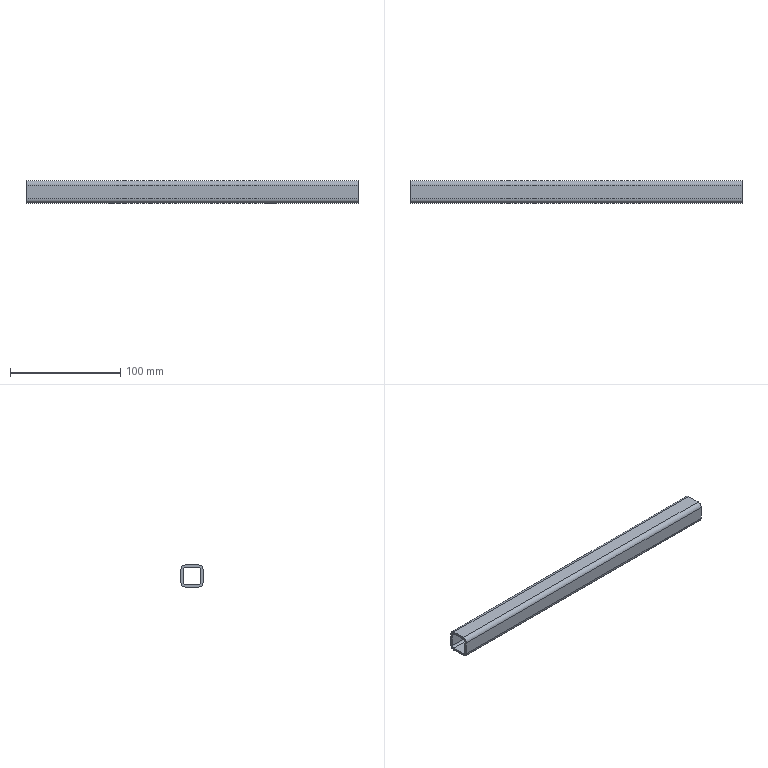Part | NX | features BREP 1 | 1 solid | 22 faces | box 300.997 x 20 x 20 mm | volume 39934 mm3 | cylinder 12 | plane 10 | commonest cylinder face diameters 4 x4 8 x4 10 x4
STEP:
#1=CARTESIAN_POINT('',(1775.533,-619.17,1465.97));
#2=VERTEX_POINT('',#1);
#3=CARTESIAN_POINT('',(1765.533,-619.17,1465.97));
#4=VERTEX_POINT('',#3);
#5=CARTESIAN_POINT('',(1775.533,-619.17,1465.97));
#6=CARTESIAN_POINT('',(1775.533,-618.622,1465.97));
#7=CARTESIAN_POINT('',(1775.458,-618.075,1465.97));
#8=CARTESIAN_POINT('',(1775.308,-617.541,1465.97));
#9=CARTESIAN_POINT('',(1774.866,-616.527,1465.97));
#10=CARTESIAN_POINT('',(1774.167,-615.67,1465.97));
#11=CARTESIAN_POINT('',(1773.761,-615.292,1465.97));
#12=CARTESIAN_POINT('',(1772.856,-614.658,1465.97));
#13=CARTESIAN_POINT('',(1771.813,-614.29,1465.97));
#14=CARTESIAN_POINT('',(1771.27,-614.179,1465.97));
#15=CARTESIAN_POINT('',(1770.166,-614.108,1465.97));
#16=CARTESIAN_POINT('',(1769.084,-614.337,1465.97));
#17=CARTESIAN_POINT('',(1768.563,-614.525,1465.97));
#18=CARTESIAN_POINT('',(1767.584,-615.04,1465.97));
#19=CARTESIAN_POINT('',(1766.78,-615.798,1465.97));
#20=CARTESIAN_POINT('',(1766.432,-616.231,1465.97));
#21=CARTESIAN_POINT('',(1765.94,-617.054,1465.97));
#22=CARTESIAN_POINT('',(1765.655,-617.967,1465.97));
#23=CARTESIAN_POINT('',(1765.574,-618.364,1465.97));
#24=CARTESIAN_POINT('',(1765.533,-618.767,1465.97));
#25=CARTESIAN_POINT('',(1765.533,-619.17,1465.97));
#26=B_SPLINE_CURVE_WITH_KNOTS('',5,(#5,#6,#7,#8,#9,#10,#11,#12,#13,#14,#15,#16,#17,#18,#19,#20,#21,#22,#23,#24,#25),.UNSPECIFIED.,.F.,.F.,(6,3,3,3,3,3,6),(0.,3.873,7.746,11.619,15.492,19.365,22.214),.UNSPECIFIED.);
#27=EDGE_CURVE('',#2,#4,#26,.T.);
#28=ORIENTED_EDGE('',*,*,#27,.F.);
#29=CARTESIAN_POINT('',(1775.533,-619.17,1467.97));
#30=VERTEX_POINT('',#29);
#31=CARTESIAN_POINT('',(1775.533,-619.17,1475.97));
#32=DIRECTION('',(0.,0.,1.));
#33=VECTOR('',#32,1000.);
#34=LINE('',#31,#33);
#35=EDGE_CURVE('',#2,#30,#34,.T.);
#36=ORIENTED_EDGE('',*,*,#35,.T.);
#37=CARTESIAN_POINT('',(1765.533,-619.17,1467.97));
#38=VERTEX_POINT('',#37);
#39=CARTESIAN_POINT('',(1775.533,-619.17,1467.97));
#40=CARTESIAN_POINT('',(1775.533,-618.622,1467.97));
#41=CARTESIAN_POINT('',(1775.458,-618.075,1467.97));
#42=CARTESIAN_POINT('',(1775.308,-617.541,1467.97));
#43=CARTESIAN_POINT('',(1774.866,-616.527,1467.97));
#44=CARTESIAN_POINT('',(1774.167,-615.67,1467.97));
#45=CARTESIAN_POINT('',(1773.761,-615.292,1467.97));
#46=CARTESIAN_POINT('',(1772.856,-614.658,1467.97));
#47=CARTESIAN_POINT('',(1771.813,-614.29,1467.97));
#48=CARTESIAN_POINT('',(1771.27,-614.179,1467.97));
#49=CARTESIAN_POINT('',(1770.166,-614.108,1467.97));
#50=CARTESIAN_POINT('',(1769.084,-614.337,1467.97));
#51=CARTESIAN_POINT('',(1768.563,-614.525,1467.97));
#52=CARTESIAN_POINT('',(1767.584,-615.04,1467.97));
#53=CARTESIAN_POINT('',(1766.78,-615.798,1467.97));
#54=CARTESIAN_POINT('',(1766.432,-616.231,1467.97));
#55=CARTESIAN_POINT('',(1765.94,-617.054,1467.97));
#56=CARTESIAN_POINT('',(1765.655,-617.967,1467.97));
#57=CARTESIAN_POINT('',(1765.574,-618.364,1467.97));
#58=CARTESIAN_POINT('',(1765.533,-618.767,1467.97));
#59=CARTESIAN_POINT('',(1765.533,-619.17,1467.97));
#60=B_SPLINE_CURVE_WITH_KNOTS('',5,(#39,#40,#41,#42,#43,#44,#45,#46,#47,#48,#49,#50,#51,#52,#53,#54,#55,#56,#57,#58,#59),.UNSPECIFIED.,.F.,.F.,(6,3,3,3,3,3,6),(0.,3.873,7.746,11.619,15.492,19.365,22.214),.UNSPECIFIED.);
#61=EDGE_CURVE('',#30,#38,#60,.T.);
#62=ORIENTED_EDGE('',*,*,#61,.T.);
#63=CARTESIAN_POINT('',(1765.533,-619.17,1475.97));
#64=DIRECTION('',(0.,0.,1.));
#65=VECTOR('',#64,1000.);
#66=LINE('',#63,#65);
#67=EDGE_CURVE('',#4,#38,#66,.T.);
#68=ORIENTED_EDGE('',*,*,#67,.F.);
#69=EDGE_LOOP('',(#28,#36,#62,#68));
#70=FACE_BOUND('',#69,.T.);
#71=CARTESIAN_POINT('',(1770.533,-619.17,1475.97));
#72=DIRECTION('',(0.,0.,1.));
#73=DIRECTION('',(1.,0.,0.));
#74=AXIS2_PLACEMENT_3D('',#71,#72,#73);
#75=CYLINDRICAL_SURFACE('',#74,5.);
#76=ADVANCED_FACE('',(#70),#75,.F.);
#77=ORIENTED_EDGE('',*,*,#35,.F.);
#78=CARTESIAN_POINT('',(1765.533,-619.17,1465.97));
#79=CARTESIAN_POINT('',(1765.533,-619.718,1465.97));
#80=CARTESIAN_POINT('',(1765.608,-620.265,1465.97));
#81=CARTESIAN_POINT('',(1765.758,-620.799,1465.97));
#82=CARTESIAN_POINT('',(1766.2,-621.813,1465.97));
#83=CARTESIAN_POINT('',(1766.899,-622.67,1465.97));
#84=CARTESIAN_POINT('',(1767.305,-623.048,1465.97));
#85=CARTESIAN_POINT('',(1768.211,-623.682,1465.97));
#86=CARTESIAN_POINT('',(1769.253,-624.05,1465.97));
#87=CARTESIAN_POINT('',(1769.797,-624.161,1465.97));
#88=CARTESIAN_POINT('',(1770.9,-624.232,1465.97));
#89=CARTESIAN_POINT('',(1771.982,-624.003,1465.97));
#90=CARTESIAN_POINT('',(1772.504,-623.815,1465.97));
#91=CARTESIAN_POINT('',(1773.482,-623.3,1465.97));
#92=CARTESIAN_POINT('',(1774.287,-622.542,1465.97));
#93=CARTESIAN_POINT('',(1774.634,-622.109,1465.97));
#94=CARTESIAN_POINT('',(1775.127,-621.286,1465.97));
#95=CARTESIAN_POINT('',(1775.411,-620.373,1465.97));
#96=CARTESIAN_POINT('',(1775.492,-619.976,1465.97));
#97=CARTESIAN_POINT('',(1775.533,-619.573,1465.97));
#98=CARTESIAN_POINT('',(1775.533,-619.17,1465.97));
#99=B_SPLINE_CURVE_WITH_KNOTS('',5,(#78,#79,#80,#81,#82,#83,#84,#85,#86,#87,#88,#89,#90,#91,#92,#93,#94,#95,#96,#97,#98),.UNSPECIFIED.,.F.,.F.,(6,3,3,3,3,3,6),(0.,3.873,7.746,11.619,15.492,19.365,22.214),.UNSPECIFIED.);
#100=EDGE_CURVE('',#4,#2,#99,.T.);
#101=ORIENTED_EDGE('',*,*,#100,.F.);
#102=ORIENTED_EDGE('',*,*,#67,.T.);
#103=CARTESIAN_POINT('',(1765.533,-619.17,1467.97));
#104=CARTESIAN_POINT('',(1765.533,-619.718,1467.97));
#105=CARTESIAN_POINT('',(1765.608,-620.265,1467.97));
#106=CARTESIAN_POINT('',(1765.758,-620.799,1467.97));
#107=CARTESIAN_POINT('',(1766.2,-621.813,1467.97));
#108=CARTESIAN_POINT('',(1766.899,-622.67,1467.97));
#109=CARTESIAN_POINT('',(1767.305,-623.048,1467.97));
#110=CARTESIAN_POINT('',(1768.211,-623.682,1467.97));
#111=CARTESIAN_POINT('',(1769.253,-624.05,1467.97));
#112=CARTESIAN_POINT('',(1769.797,-624.161,1467.97));
#113=CARTESIAN_POINT('',(1770.9,-624.232,1467.97));
#114=CARTESIAN_POINT('',(1771.982,-624.003,1467.97));
#115=CARTESIAN_POINT('',(1772.504,-623.815,1467.97));
#116=CARTESIAN_POINT('',(1773.482,-623.3,1467.97));
#117=CARTESIAN_POINT('',(1774.287,-622.542,1467.97));
#118=CARTESIAN_POINT('',(1774.634,-622.109,1467.97));
#119=CARTESIAN_POINT('',(1775.127,-621.286,1467.97));
#120=CARTESIAN_POINT('',(1775.411,-620.373,1467.97));
#121=CARTESIAN_POINT('',(1775.492,-619.976,1467.97));
#122=CARTESIAN_POINT('',(1775.533,-619.573,1467.97));
#123=CARTESIAN_POINT('',(1775.533,-619.17,1467.97));
#124=B_SPLINE_CURVE_WITH_KNOTS('',5,(#103,#104,#105,#106,#107,#108,#109,#110,#111,#112,#113,#114,#115,#116,#117,#118,#119,#120,#121,#122,#123),.UNSPECIFIED.,.F.,.F.,(6,3,3,3,3,3,6),(0.,3.873,7.746,11.619,15.492,19.365,22.214),.UNSPECIFIED.);
#125=EDGE_CURVE('',#38,#30,#124,.T.);
#126=ORIENTED_EDGE('',*,*,#125,.T.);
#127=EDGE_LOOP('',(#77,#101,#102,#126));
#128=FACE_BOUND('',#127,.T.);
#129=CARTESIAN_POINT('',(1770.533,-619.17,1475.97));
#130=DIRECTION('',(0.,0.,1.));
#131=DIRECTION('',(-1.,0.,0.));
#132=AXIS2_PLACEMENT_3D('',#129,#130,#131);
#133=CYLINDRICAL_SURFACE('',#132,5.);
#134=ADVANCED_FACE('',(#128),#133,.F.);
#135=CARTESIAN_POINT('',(1634.544,-619.17,1467.97));
#136=VERTEX_POINT('',#135);
#137=CARTESIAN_POINT('',(1634.544,-619.17,1465.97));
#138=VERTEX_POINT('',#137);
#139=CARTESIAN_POINT('',(1634.544,-619.17,1475.97));
#140=DIRECTION('',(0.,0.,-1.));
#141=VECTOR('',#140,1000.);
#142=LINE('',#139,#141);
#143=EDGE_CURVE('',#136,#138,#142,.T.);
#144=ORIENTED_EDGE('',*,*,#143,.F.);
#145=CARTESIAN_POINT('',(1624.544,-619.17,1467.97));
#146=VERTEX_POINT('',#145);
#147=CARTESIAN_POINT('',(1629.544,-619.17,1467.97));
#148=DIRECTION('',(0.,0.,-1.));
#149=DIRECTION('',(-1.,0.,0.));
#150=AXIS2_PLACEMENT_3D('',#147,#148,#149);
#151=CIRCLE('',#150,5.);
#152=EDGE_CURVE('',#146,#136,#151,.T.);
#153=ORIENTED_EDGE('',*,*,#152,.F.);
#154=CARTESIAN_POINT('',(1624.544,-619.17,1465.97));
#155=VERTEX_POINT('',#154);
#156=CARTESIAN_POINT('',(1624.544,-619.17,1475.97));
#157=DIRECTION('',(0.,0.,-1.));
#158=VECTOR('',#157,1000.);
#159=LINE('',#156,#158);
#160=EDGE_CURVE('',#146,#155,#159,.T.);
#161=ORIENTED_EDGE('',*,*,#160,.T.);
#162=CARTESIAN_POINT('',(1629.544,-619.17,1465.97));
#163=DIRECTION('',(0.,0.,-1.));
#164=DIRECTION('',(-1.,0.,0.));
#165=AXIS2_PLACEMENT_3D('',#162,#163,#164);
#166=CIRCLE('',#165,5.);
#167=EDGE_CURVE('',#155,#138,#166,.T.);
#168=ORIENTED_EDGE('',*,*,#167,.T.);
#169=EDGE_LOOP('',(#144,#153,#161,#168));
#170=FACE_BOUND('',#169,.T.);
#171=CARTESIAN_POINT('',(1629.544,-619.17,1475.97));
#172=DIRECTION('',(0.,0.,-1.));
#173=DIRECTION('',(-1.,0.,0.));
#174=AXIS2_PLACEMENT_3D('',#171,#172,#173);
#175=CYLINDRICAL_SURFACE('',#174,5.);
#176=ADVANCED_FACE('',(#170),#175,.F.);
#177=CARTESIAN_POINT('',(1629.544,-619.17,1467.97));
#178=DIRECTION('',(0.,0.,-1.));
#179=DIRECTION('',(-1.,0.,0.));
#180=AXIS2_PLACEMENT_3D('',#177,#178,#179);
#181=CIRCLE('',#180,5.);
#182=EDGE_CURVE('',#136,#146,#181,.T.);
#183=ORIENTED_EDGE('',*,*,#182,.F.);
#184=ORIENTED_EDGE('',*,*,#143,.T.);
#185=CARTESIAN_POINT('',(1629.544,-619.17,1465.97));
#186=DIRECTION('',(0.,0.,-1.));
#187=DIRECTION('',(-1.,0.,0.));
#188=AXIS2_PLACEMENT_3D('',#185,#186,#187);
#189=CIRCLE('',#188,5.);
#190=EDGE_CURVE('',#138,#155,#189,.T.);
#191=ORIENTED_EDGE('',*,*,#190,.T.);
#192=ORIENTED_EDGE('',*,*,#160,.F.);
#193=EDGE_LOOP('',(#183,#184,#191,#192));
#194=FACE_BOUND('',#193,.T.);
#195=CARTESIAN_POINT('',(1629.544,-619.17,1475.97));
#196=DIRECTION('',(0.,0.,-1.));
#197=DIRECTION('',(1.,0.,0.));
#198=AXIS2_PLACEMENT_3D('',#195,#196,#197);
#199=CYLINDRICAL_SURFACE('',#198,5.);
#200=ADVANCED_FACE('',(#194),#199,.F.);
#201=CARTESIAN_POINT('',(1549.54,-613.17,1467.97));
#202=VERTEX_POINT('',#201);
#203=CARTESIAN_POINT('',(1549.54,-611.17,1469.97));
#204=VERTEX_POINT('',#203);
#205=CARTESIAN_POINT('',(1549.54,-613.17,1469.97));
#206=DIRECTION('',(1.,0.,0.));
#207=DIRECTION('',(0.,0.,-1.));
#208=AXIS2_PLACEMENT_3D('',#205,#206,#207);
#209=CIRCLE('',#208,2.);
#210=EDGE_CURVE('',#202,#204,#209,.T.);
#211=ORIENTED_EDGE('',*,*,#210,.T.);
#212=CARTESIAN_POINT('',(1549.54,-611.17,1481.97));
#213=VERTEX_POINT('',#212);
#214=CARTESIAN_POINT('',(1549.54,-611.17,1475.97));
#215=DIRECTION('',(0.,0.,-1.));
#216=VECTOR('',#215,1000.);
#217=LINE('',#214,#216);
#218=EDGE_CURVE('',#213,#204,#217,.T.);
#219=ORIENTED_EDGE('',*,*,#218,.F.);
#220=CARTESIAN_POINT('',(1549.54,-613.17,1483.97));
#221=VERTEX_POINT('',#220);
#222=CARTESIAN_POINT('',(1549.54,-613.17,1481.97));
#223=DIRECTION('',(1.,0.,0.));
#224=DIRECTION('',(0.,0.,-1.));
#225=AXIS2_PLACEMENT_3D('',#222,#223,#224);
#226=CIRCLE('',#225,2.);
#227=EDGE_CURVE('',#213,#221,#226,.T.);
#228=ORIENTED_EDGE('',*,*,#227,.T.);
#229=CARTESIAN_POINT('',(1549.54,-625.17,1483.97));
#230=VERTEX_POINT('',#229);
#231=CARTESIAN_POINT('',(1549.54,-619.17,1483.97));
#232=DIRECTION('',(0.,-1.,0.));
#233=VECTOR('',#232,1000.);
#234=LINE('',#231,#233);
#235=EDGE_CURVE('',#221,#230,#234,.T.);
#236=ORIENTED_EDGE('',*,*,#235,.T.);
#237=CARTESIAN_POINT('',(1549.54,-627.17,1481.97));
#238=VERTEX_POINT('',#237);
#239=CARTESIAN_POINT('',(1549.54,-625.17,1481.97));
#240=DIRECTION('',(1.,0.,0.));
#241=DIRECTION('',(0.,0.,-1.));
#242=AXIS2_PLACEMENT_3D('',#239,#240,#241);
#243=CIRCLE('',#242,2.);
#244=EDGE_CURVE('',#230,#238,#243,.T.);
#245=ORIENTED_EDGE('',*,*,#244,.T.);
#246=CARTESIAN_POINT('',(1549.54,-627.17,1469.97));
#247=VERTEX_POINT('',#246);
#248=CARTESIAN_POINT('',(1549.54,-627.17,1475.97));
#249=DIRECTION('',(0.,0.,-1.));
#250=VECTOR('',#249,1000.);
#251=LINE('',#248,#250);
#252=EDGE_CURVE('',#238,#247,#251,.T.);
#253=ORIENTED_EDGE('',*,*,#252,.T.);
#254=CARTESIAN_POINT('',(1549.54,-625.17,1467.97));
#255=VERTEX_POINT('',#254);
#256=CARTESIAN_POINT('',(1549.54,-625.17,1469.97));
#257=DIRECTION('',(1.,0.,0.));
#258=DIRECTION('',(0.,0.,-1.));
#259=AXIS2_PLACEMENT_3D('',#256,#257,#258);
#260=CIRCLE('',#259,2.);
#261=EDGE_CURVE('',#247,#255,#260,.T.);
#262=ORIENTED_EDGE('',*,*,#261,.T.);
#263=CARTESIAN_POINT('',(1549.54,-619.17,1467.97));
#264=DIRECTION('',(0.,-1.,0.));
#265=VECTOR('',#264,1000.);
#266=LINE('',#263,#265);
#267=EDGE_CURVE('',#202,#255,#266,.T.);
#268=ORIENTED_EDGE('',*,*,#267,.F.);
#269=EDGE_LOOP('',(#211,#219,#228,#236,#245,#253,#262,#268));
#270=FACE_BOUND('',#269,.T.);
#271=CARTESIAN_POINT('',(1549.54,-629.17,1469.97));
#272=VERTEX_POINT('',#271);
#273=CARTESIAN_POINT('',(1549.54,-625.17,1465.97));
#274=VERTEX_POINT('',#273);
#275=CARTESIAN_POINT('',(1549.54,-625.17,1469.97));
#276=DIRECTION('',(1.,0.,0.));
#277=DIRECTION('',(0.,0.,-1.));
#278=AXIS2_PLACEMENT_3D('',#275,#276,#277);
#279=CIRCLE('',#278,4.);
#280=EDGE_CURVE('',#272,#274,#279,.T.);
#281=ORIENTED_EDGE('',*,*,#280,.F.);
#282=CARTESIAN_POINT('',(1549.54,-629.17,1481.97));
#283=VERTEX_POINT('',#282);
#284=CARTESIAN_POINT('',(1549.54,-629.17,1475.97));
#285=DIRECTION('',(0.,0.,-1.));
#286=VECTOR('',#285,1000.);
#287=LINE('',#284,#286);
#288=EDGE_CURVE('',#283,#272,#287,.T.);
#289=ORIENTED_EDGE('',*,*,#288,.F.);
#290=CARTESIAN_POINT('',(1549.54,-625.17,1485.97));
#291=VERTEX_POINT('',#290);
#292=CARTESIAN_POINT('',(1549.54,-625.17,1481.97));
#293=DIRECTION('',(1.,0.,0.));
#294=DIRECTION('',(0.,0.,-1.));
#295=AXIS2_PLACEMENT_3D('',#292,#293,#294);
#296=CIRCLE('',#295,4.);
#297=EDGE_CURVE('',#291,#283,#296,.T.);
#298=ORIENTED_EDGE('',*,*,#297,.F.);
#299=CARTESIAN_POINT('',(1549.54,-613.17,1485.97));
#300=VERTEX_POINT('',#299);
#301=CARTESIAN_POINT('',(1549.54,-619.17,1485.97));
#302=DIRECTION('',(0.,-1.,0.));
#303=VECTOR('',#302,1000.);
#304=LINE('',#301,#303);
#305=EDGE_CURVE('',#300,#291,#304,.T.);
#306=ORIENTED_EDGE('',*,*,#305,.F.);
#307=CARTESIAN_POINT('',(1549.54,-609.17,1481.97));
#308=VERTEX_POINT('',#307);
#309=CARTESIAN_POINT('',(1549.54,-613.17,1481.97));
#310=DIRECTION('',(1.,0.,0.));
#311=DIRECTION('',(0.,0.,-1.));
#312=AXIS2_PLACEMENT_3D('',#309,#310,#311);
#313=CIRCLE('',#312,4.);
#314=EDGE_CURVE('',#308,#300,#313,.T.);
#315=ORIENTED_EDGE('',*,*,#314,.F.);
#316=CARTESIAN_POINT('',(1549.54,-609.17,1469.97));
#317=VERTEX_POINT('',#316);
#318=CARTESIAN_POINT('',(1549.54,-609.17,1475.97));
#319=DIRECTION('',(0.,0.,-1.));
#320=VECTOR('',#319,1000.);
#321=LINE('',#318,#320);
#322=EDGE_CURVE('',#308,#317,#321,.T.);
#323=ORIENTED_EDGE('',*,*,#322,.T.);
#324=CARTESIAN_POINT('',(1549.54,-613.17,1465.97));
#325=VERTEX_POINT('',#324);
#326=CARTESIAN_POINT('',(1549.54,-613.17,1469.97));
#327=DIRECTION('',(1.,0.,0.));
#328=DIRECTION('',(0.,0.,-1.));
#329=AXIS2_PLACEMENT_3D('',#326,#327,#328);
#330=CIRCLE('',#329,4.);
#331=EDGE_CURVE('',#325,#317,#330,.T.);
#332=ORIENTED_EDGE('',*,*,#331,.F.);
#333=CARTESIAN_POINT('',(1549.54,-619.17,1465.97));
#334=DIRECTION('',(0.,-1.,0.));
#335=VECTOR('',#334,1000.);
#336=LINE('',#333,#335);
#337=EDGE_CURVE('',#325,#274,#336,.T.);
#338=ORIENTED_EDGE('',*,*,#337,.T.);
#339=EDGE_LOOP('',(#281,#289,#298,#306,#315,#323,#332,#338));
#340=FACE_BOUND('',#339,.T.);
#341=CARTESIAN_POINT('',(1549.54,-314.585,1465.97));
#342=DIRECTION('',(-1.,0.,0.));
#343=DIRECTION('',(0.,0.,1.));
#344=AXIS2_PLACEMENT_3D('',#341,#342,#343);
#345=PLANE('',#344);
#346=ADVANCED_FACE('',(#270,#340),#345,.T.);
#347=ORIENTED_EDGE('',*,*,#210,.F.);
#348=CARTESIAN_POINT('',(1850.537,-613.17,1467.97));
#349=VERTEX_POINT('',#348);
#350=CARTESIAN_POINT('',(1700.039,-613.17,1467.97));
#351=DIRECTION('',(1.,0.,0.));
#352=VECTOR('',#351,1000.);
#353=LINE('',#350,#352);
#354=EDGE_CURVE('',#202,#349,#353,.T.);
#355=ORIENTED_EDGE('',*,*,#354,.T.);
#356=CARTESIAN_POINT('',(1850.537,-611.17,1469.97));
#357=VERTEX_POINT('',#356);
#358=CARTESIAN_POINT('',(1850.537,-611.17,1469.97));
#359=CARTESIAN_POINT('',(1850.537,-611.17,1468.91));
#360=CARTESIAN_POINT('',(1850.537,-612.108,1467.97));
#361=CARTESIAN_POINT('',(1850.537,-613.17,1467.97));
#362=B_SPLINE_CURVE_WITH_KNOTS('',3,(#358,#359,#360,#361),.UNSPECIFIED.,.F.,.F.,(4,4),(0.,1.),.UNSPECIFIED.);
#363=EDGE_CURVE('',#357,#349,#362,.T.);
#364=ORIENTED_EDGE('',*,*,#363,.F.);
#365=CARTESIAN_POINT('',(1700.039,-611.17,1469.97));
#366=DIRECTION('',(1.,0.,0.));
#367=VECTOR('',#366,1000.);
#368=LINE('',#365,#367);
#369=EDGE_CURVE('',#204,#357,#368,.T.);
#370=ORIENTED_EDGE('',*,*,#369,.F.);
#371=EDGE_LOOP('',(#347,#355,#364,#370));
#372=FACE_BOUND('',#371,.T.);
#373=CARTESIAN_POINT('',(502.707,-613.17,1469.97));
#374=DIRECTION('',(1.,0.,0.));
#375=DIRECTION('',(0.,-1.,0.));
#376=AXIS2_PLACEMENT_3D('',#373,#374,#375);
#377=CYLINDRICAL_SURFACE('',#376,2.);
#378=ADVANCED_FACE('',(#372),#377,.F.);
#379=ORIENTED_EDGE('',*,*,#218,.T.);
#380=ORIENTED_EDGE('',*,*,#369,.T.);
#381=CARTESIAN_POINT('',(1850.537,-611.17,1481.97));
#382=VERTEX_POINT('',#381);
#383=CARTESIAN_POINT('',(1850.537,-611.17,1475.97));
#384=DIRECTION('',(0.,0.,1.));
#385=VECTOR('',#384,1000.);
#386=LINE('',#383,#385);
#387=EDGE_CURVE('',#357,#382,#386,.T.);
#388=ORIENTED_EDGE('',*,*,#387,.T.);
#389=CARTESIAN_POINT('',(502.707,-611.17,1481.97));
#390=DIRECTION('',(1.,0.,0.));
#391=VECTOR('',#390,1000.);
#392=LINE('',#389,#391);
#393=EDGE_CURVE('',#213,#382,#392,.T.);
#394=ORIENTED_EDGE('',*,*,#393,.F.);
#395=EDGE_LOOP('',(#379,#380,#388,#394));
#396=FACE_BOUND('',#395,.T.);
#397=CARTESIAN_POINT('',(502.707,-611.17,1469.97));
#398=DIRECTION('',(0.,1.,0.));
#399=DIRECTION('',(-1.,0.,0.));
#400=AXIS2_PLACEMENT_3D('',#397,#398,#399);
#401=PLANE('',#400);
#402=ADVANCED_FACE('',(#396),#401,.F.);
#403=ORIENTED_EDGE('',*,*,#227,.F.);
#404=ORIENTED_EDGE('',*,*,#393,.T.);
#405=CARTESIAN_POINT('',(1850.537,-613.17,1483.97));
#406=VERTEX_POINT('',#405);
#407=CARTESIAN_POINT('',(1850.537,-613.17,1483.97));
#408=CARTESIAN_POINT('',(1850.537,-612.109,1483.97));
#409=CARTESIAN_POINT('',(1850.537,-611.17,1483.033));
#410=CARTESIAN_POINT('',(1850.537,-611.17,1481.97));
#411=B_SPLINE_CURVE_WITH_KNOTS('',3,(#407,#408,#409,#410),.UNSPECIFIED.,.F.,.F.,(4,4),(0.,1.),.UNSPECIFIED.);
#412=EDGE_CURVE('',#406,#382,#411,.T.);
#413=ORIENTED_EDGE('',*,*,#412,.F.);
#414=CARTESIAN_POINT('',(1700.039,-613.17,1483.97));
#415=DIRECTION('',(1.,0.,0.));
#416=VECTOR('',#415,1000.);
#417=LINE('',#414,#416);
#418=EDGE_CURVE('',#221,#406,#417,.T.);
#419=ORIENTED_EDGE('',*,*,#418,.F.);
#420=EDGE_LOOP('',(#403,#404,#413,#419));
#421=FACE_BOUND('',#420,.T.);
#422=CARTESIAN_POINT('',(502.707,-613.17,1481.97));
#423=DIRECTION('',(1.,0.,0.));
#424=DIRECTION('',(0.,1.,0.));
#425=AXIS2_PLACEMENT_3D('',#422,#423,#424);
#426=CYLINDRICAL_SURFACE('',#425,2.);
#427=ADVANCED_FACE('',(#421),#426,.F.);
#428=ORIENTED_EDGE('',*,*,#235,.F.);
#429=ORIENTED_EDGE('',*,*,#418,.T.);
#430=CARTESIAN_POINT('',(1850.537,-625.17,1483.97));
#431=VERTEX_POINT('',#430);
#432=CARTESIAN_POINT('',(1850.537,-619.17,1483.97));
#433=DIRECTION('',(0.,1.,0.));
#434=VECTOR('',#433,1000.);
#435=LINE('',#432,#434);
#436=EDGE_CURVE('',#431,#406,#435,.T.);
#437=ORIENTED_EDGE('',*,*,#436,.F.);
#438=CARTESIAN_POINT('',(502.707,-625.17,1483.97));
#439=DIRECTION('',(1.,0.,0.));
#440=VECTOR('',#439,1000.);
#441=LINE('',#438,#440);
#442=EDGE_CURVE('',#230,#431,#441,.T.);
#443=ORIENTED_EDGE('',*,*,#442,.F.);
#444=EDGE_LOOP('',(#428,#429,#437,#443));
#445=FACE_BOUND('',#444,.T.);
#446=CARTESIAN_POINT('',(502.707,-613.17,1483.97));
#447=DIRECTION('',(0.,0.,1.));
#448=DIRECTION('',(1.,0.,0.));
#449=AXIS2_PLACEMENT_3D('',#446,#447,#448);
#450=PLANE('',#449);
#451=ADVANCED_FACE('',(#445),#450,.F.);
#452=ORIENTED_EDGE('',*,*,#244,.F.);
#453=ORIENTED_EDGE('',*,*,#442,.T.);
#454=CARTESIAN_POINT('',(1850.537,-627.17,1481.97));
#455=VERTEX_POINT('',#454);
#456=CARTESIAN_POINT('',(1850.537,-627.17,1481.97));
#457=CARTESIAN_POINT('',(1850.537,-627.17,1483.031));
#458=CARTESIAN_POINT('',(1850.537,-626.232,1483.97));
#459=CARTESIAN_POINT('',(1850.537,-625.17,1483.97));
#460=B_SPLINE_CURVE_WITH_KNOTS('',3,(#456,#457,#458,#459),.UNSPECIFIED.,.F.,.F.,(4,4),(0.,1.),.UNSPECIFIED.);
#461=EDGE_CURVE('',#455,#431,#460,.T.);
#462=ORIENTED_EDGE('',*,*,#461,.F.);
#463=CARTESIAN_POINT('',(1700.039,-627.17,1481.97));
#464=DIRECTION('',(1.,0.,0.));
#465=VECTOR('',#464,1000.);
#466=LINE('',#463,#465);
#467=EDGE_CURVE('',#238,#455,#466,.T.);
#468=ORIENTED_EDGE('',*,*,#467,.F.);
#469=EDGE_LOOP('',(#452,#453,#462,#468));
#470=FACE_BOUND('',#469,.T.);
#471=CARTESIAN_POINT('',(502.707,-625.17,1481.97));
#472=DIRECTION('',(1.,0.,0.));
#473=DIRECTION('',(0.,1.,0.));
#474=AXIS2_PLACEMENT_3D('',#471,#472,#473);
#475=CYLINDRICAL_SURFACE('',#474,2.);
#476=ADVANCED_FACE('',(#470),#475,.F.);
#477=ORIENTED_EDGE('',*,*,#252,.F.);
#478=ORIENTED_EDGE('',*,*,#467,.T.);
#479=CARTESIAN_POINT('',(1850.537,-627.17,1469.97));
#480=VERTEX_POINT('',#479);
#481=CARTESIAN_POINT('',(1850.537,-627.17,1475.97));
#482=DIRECTION('',(0.,0.,1.));
#483=VECTOR('',#482,1000.);
#484=LINE('',#481,#483);
#485=EDGE_CURVE('',#480,#455,#484,.T.);
#486=ORIENTED_EDGE('',*,*,#485,.F.);
#487=CARTESIAN_POINT('',(502.707,-627.17,1469.97));
#488=DIRECTION('',(1.,0.,0.));
#489=VECTOR('',#488,1000.);
#490=LINE('',#487,#489);
#491=EDGE_CURVE('',#247,#480,#490,.T.);
#492=ORIENTED_EDGE('',*,*,#491,.F.);
#493=EDGE_LOOP('',(#477,#478,#486,#492));
#494=FACE_BOUND('',#493,.T.);
#495=CARTESIAN_POINT('',(502.707,-627.17,1481.97));
#496=DIRECTION('',(0.,-1.,0.));
#497=DIRECTION('',(1.,0.,0.));
#498=AXIS2_PLACEMENT_3D('',#495,#496,#497);
#499=PLANE('',#498);
#500=ADVANCED_FACE('',(#494),#499,.F.);
#501=ORIENTED_EDGE('',*,*,#261,.F.);
#502=ORIENTED_EDGE('',*,*,#491,.T.);
#503=CARTESIAN_POINT('',(1850.537,-625.17,1467.97));
#504=VERTEX_POINT('',#503);
#505=CARTESIAN_POINT('',(1850.537,-625.17,1467.97));
#506=CARTESIAN_POINT('',(1850.537,-626.231,1467.97));
#507=CARTESIAN_POINT('',(1850.537,-627.17,1468.908));
#508=CARTESIAN_POINT('',(1850.537,-627.17,1469.97));
#509=B_SPLINE_CURVE_WITH_KNOTS('',3,(#505,#506,#507,#508),.UNSPECIFIED.,.F.,.F.,(4,4),(0.,1.),.UNSPECIFIED.);
#510=EDGE_CURVE('',#504,#480,#509,.T.);
#511=ORIENTED_EDGE('',*,*,#510,.F.);
#512=CARTESIAN_POINT('',(1700.039,-625.17,1467.97));
#513=DIRECTION('',(1.,0.,0.));
#514=VECTOR('',#513,1000.);
#515=LINE('',#512,#514);
#516=EDGE_CURVE('',#255,#504,#515,.T.);
#517=ORIENTED_EDGE('',*,*,#516,.F.);
#518=EDGE_LOOP('',(#501,#502,#511,#517));
#519=FACE_BOUND('',#518,.T.);
#520=CARTESIAN_POINT('',(502.707,-625.17,1469.97));
#521=DIRECTION('',(1.,0.,0.));
#522=DIRECTION('',(0.,-1.,0.));
#523=AXIS2_PLACEMENT_3D('',#520,#521,#522);
#524=CYLINDRICAL_SURFACE('',#523,2.);
#525=ADVANCED_FACE('',(#519),#524,.F.);
#526=ORIENTED_EDGE('',*,*,#61,.F.);
#527=ORIENTED_EDGE('',*,*,#125,.F.);
#528=EDGE_LOOP('',(#526,#527));
#529=FACE_BOUND('',#528,.T.);
#530=ORIENTED_EDGE('',*,*,#182,.T.);
#531=ORIENTED_EDGE('',*,*,#152,.T.);
#532=EDGE_LOOP('',(#530,#531));
#533=FACE_BOUND('',#532,.T.);
#534=ORIENTED_EDGE('',*,*,#267,.T.);
#535=ORIENTED_EDGE('',*,*,#516,.T.);
#536=CARTESIAN_POINT('',(1850.537,-619.17,1467.97));
#537=DIRECTION('',(0.,1.,0.));
#538=VECTOR('',#537,1000.);
#539=LINE('',#536,#538);
#540=EDGE_CURVE('',#504,#349,#539,.T.);
#541=ORIENTED_EDGE('',*,*,#540,.T.);
#542=ORIENTED_EDGE('',*,*,#354,.F.);
#543=EDGE_LOOP('',(#534,#535,#541,#542));
#544=FACE_BOUND('',#543,.T.);
#545=CARTESIAN_POINT('',(502.707,-625.17,1467.97));
#546=DIRECTION('',(0.,0.,-1.));
#547=DIRECTION('',(-1.,0.,0.));
#548=AXIS2_PLACEMENT_3D('',#545,#546,#547);
#549=PLANE('',#548);
#550=ADVANCED_FACE('',(#529,#533,#544),#549,.F.);
#551=ORIENTED_EDGE('',*,*,#100,.T.);
#552=ORIENTED_EDGE('',*,*,#27,.T.);
#553=EDGE_LOOP('',(#551,#552));
#554=FACE_BOUND('',#553,.T.);
#555=ORIENTED_EDGE('',*,*,#190,.F.);
#556=ORIENTED_EDGE('',*,*,#167,.F.);
#557=EDGE_LOOP('',(#555,#556));
#558=FACE_BOUND('',#557,.T.);
#559=CARTESIAN_POINT('',(1850.537,-613.17,1465.97));
#560=VERTEX_POINT('',#559);
#561=CARTESIAN_POINT('',(502.707,-613.17,1465.97));
#562=DIRECTION('',(1.,0.,0.));
#563=VECTOR('',#562,1000.);
#564=LINE('',#561,#563);
#565=EDGE_CURVE('',#325,#560,#564,.T.);
#566=ORIENTED_EDGE('',*,*,#565,.T.);
#567=CARTESIAN_POINT('',(1850.537,-625.17,1465.97));
#568=VERTEX_POINT('',#567);
#569=CARTESIAN_POINT('',(1850.537,-619.17,1465.97));
#570=DIRECTION('',(0.,1.,0.));
#571=VECTOR('',#570,1000.);
#572=LINE('',#569,#571);
#573=EDGE_CURVE('',#568,#560,#572,.T.);
#574=ORIENTED_EDGE('',*,*,#573,.F.);
#575=CARTESIAN_POINT('',(502.707,-625.17,1465.97));
#576=DIRECTION('',(1.,0.,0.));
#577=VECTOR('',#576,1000.);
#578=LINE('',#575,#577);
#579=EDGE_CURVE('',#274,#568,#578,.T.);
#580=ORIENTED_EDGE('',*,*,#579,.F.);
#581=ORIENTED_EDGE('',*,*,#337,.F.);
#582=EDGE_LOOP('',(#566,#574,#580,#581));
#583=FACE_BOUND('',#582,.T.);
#584=CARTESIAN_POINT('',(502.707,-625.17,1465.97));
#585=DIRECTION('',(0.,0.,-1.));
#586=DIRECTION('',(-1.,0.,0.));
#587=AXIS2_PLACEMENT_3D('',#584,#585,#586);
#588=PLANE('',#587);
#589=ADVANCED_FACE('',(#554,#558,#583),#588,.T.);
#590=ORIENTED_EDGE('',*,*,#579,.T.);
#591=CARTESIAN_POINT('',(1850.537,-629.17,1469.97));
#592=VERTEX_POINT('',#591);
#593=CARTESIAN_POINT('',(1850.537,-629.17,1469.97));
#594=CARTESIAN_POINT('',(1850.537,-629.17,1468.92));
#595=CARTESIAN_POINT('',(1850.537,-628.301,1466.839));
#596=CARTESIAN_POINT('',(1850.537,-626.222,1465.97));
#597=CARTESIAN_POINT('',(1850.537,-625.17,1465.97));
#598=B_SPLINE_CURVE_WITH_KNOTS('',3,(#593,#594,#595,#596,#597),.UNSPECIFIED.,.F.,.F.,(4,1,4),(0.,0.5,1.),.UNSPECIFIED.);
#599=EDGE_CURVE('',#568,#592,#598,.F.);
#600=ORIENTED_EDGE('',*,*,#599,.T.);
#601=CARTESIAN_POINT('',(1700.039,-629.17,1469.97));
#602=DIRECTION('',(1.,0.,0.));
#603=VECTOR('',#602,1000.);
#604=LINE('',#601,#603);
#605=EDGE_CURVE('',#272,#592,#604,.T.);
#606=ORIENTED_EDGE('',*,*,#605,.F.);
#607=ORIENTED_EDGE('',*,*,#280,.T.);
#608=EDGE_LOOP('',(#590,#600,#606,#607));
#609=FACE_BOUND('',#608,.T.);
#610=CARTESIAN_POINT('',(502.707,-625.17,1469.97));
#611=DIRECTION('',(1.,0.,0.));
#612=DIRECTION('',(0.,-1.,0.));
#613=AXIS2_PLACEMENT_3D('',#610,#611,#612);
#614=CYLINDRICAL_SURFACE('',#613,4.);
#615=ADVANCED_FACE('',(#609),#614,.T.);
#616=ORIENTED_EDGE('',*,*,#605,.T.);
#617=CARTESIAN_POINT('',(1850.537,-629.17,1481.97));
#618=VERTEX_POINT('',#617);
#619=CARTESIAN_POINT('',(1850.537,-629.17,1475.97));
#620=DIRECTION('',(0.,0.,1.));
#621=VECTOR('',#620,1000.);
#622=LINE('',#619,#621);
#623=EDGE_CURVE('',#592,#618,#622,.T.);
#624=ORIENTED_EDGE('',*,*,#623,.T.);
#625=CARTESIAN_POINT('',(502.707,-629.17,1481.97));
#626=DIRECTION('',(1.,0.,0.));
#627=VECTOR('',#626,1000.);
#628=LINE('',#625,#627);
#629=EDGE_CURVE('',#283,#618,#628,.T.);
#630=ORIENTED_EDGE('',*,*,#629,.F.);
#631=ORIENTED_EDGE('',*,*,#288,.T.);
#632=EDGE_LOOP('',(#616,#624,#630,#631));
#633=FACE_BOUND('',#632,.T.);
#634=CARTESIAN_POINT('',(502.707,-629.17,1481.97));
#635=DIRECTION('',(0.,-1.,0.));
#636=DIRECTION('',(1.,0.,0.));
#637=AXIS2_PLACEMENT_3D('',#634,#635,#636);
#638=PLANE('',#637);
#639=ADVANCED_FACE('',(#633),#638,.T.);
#640=ORIENTED_EDGE('',*,*,#629,.T.);
#641=CARTESIAN_POINT('',(1850.537,-625.17,1485.97));
#642=VERTEX_POINT('',#641);
#643=CARTESIAN_POINT('',(1850.537,-625.17,1485.97));
#644=CARTESIAN_POINT('',(1850.537,-626.221,1485.97));
#645=CARTESIAN_POINT('',(1850.537,-628.301,1485.101));
#646=CARTESIAN_POINT('',(1850.537,-629.17,1483.022));
#647=CARTESIAN_POINT('',(1850.537,-629.17,1481.97));
#648=B_SPLINE_CURVE_WITH_KNOTS('',3,(#643,#644,#645,#646,#647),.UNSPECIFIED.,.F.,.F.,(4,1,4),(0.,0.5,1.),.UNSPECIFIED.);
#649=EDGE_CURVE('',#618,#642,#648,.F.);
#650=ORIENTED_EDGE('',*,*,#649,.T.);
#651=CARTESIAN_POINT('',(1700.039,-625.17,1485.97));
#652=DIRECTION('',(1.,0.,0.));
#653=VECTOR('',#652,1000.);
#654=LINE('',#651,#653);
#655=EDGE_CURVE('',#291,#642,#654,.T.);
#656=ORIENTED_EDGE('',*,*,#655,.F.);
#657=ORIENTED_EDGE('',*,*,#297,.T.);
#658=EDGE_LOOP('',(#640,#650,#656,#657));
#659=FACE_BOUND('',#658,.T.);
#660=CARTESIAN_POINT('',(502.707,-625.17,1481.97));
#661=DIRECTION('',(1.,0.,0.));
#662=DIRECTION('',(0.,1.,0.));
#663=AXIS2_PLACEMENT_3D('',#660,#661,#662);
#664=CYLINDRICAL_SURFACE('',#663,4.);
#665=ADVANCED_FACE('',(#659),#664,.T.);
#666=ORIENTED_EDGE('',*,*,#655,.T.);
#667=CARTESIAN_POINT('',(1850.537,-613.17,1485.97));
#668=VERTEX_POINT('',#667);
#669=CARTESIAN_POINT('',(1850.537,-619.17,1485.97));
#670=DIRECTION('',(0.,1.,0.));
#671=VECTOR('',#670,1000.);
#672=LINE('',#669,#671);
#673=EDGE_CURVE('',#642,#668,#672,.T.);
#674=ORIENTED_EDGE('',*,*,#673,.T.);
#675=CARTESIAN_POINT('',(502.707,-613.17,1485.97));
#676=DIRECTION('',(1.,0.,0.));
#677=VECTOR('',#676,1000.);
#678=LINE('',#675,#677);
#679=EDGE_CURVE('',#300,#668,#678,.T.);
#680=ORIENTED_EDGE('',*,*,#679,.F.);
#681=ORIENTED_EDGE('',*,*,#305,.T.);
#682=EDGE_LOOP('',(#666,#674,#680,#681));
#683=FACE_BOUND('',#682,.T.);
#684=CARTESIAN_POINT('',(502.707,-613.17,1485.97));
#685=DIRECTION('',(0.,0.,1.));
#686=DIRECTION('',(1.,0.,0.));
#687=AXIS2_PLACEMENT_3D('',#684,#685,#686);
#688=PLANE('',#687);
#689=ADVANCED_FACE('',(#683),#688,.T.);
#690=ORIENTED_EDGE('',*,*,#679,.T.);
#691=CARTESIAN_POINT('',(1850.537,-609.17,1481.97));
#692=VERTEX_POINT('',#691);
#693=CARTESIAN_POINT('',(1850.537,-609.17,1481.97));
#694=CARTESIAN_POINT('',(1850.537,-609.17,1483.021));
#695=CARTESIAN_POINT('',(1850.537,-610.039,1485.102));
#696=CARTESIAN_POINT('',(1850.537,-612.118,1485.97));
#697=CARTESIAN_POINT('',(1850.537,-613.17,1485.97));
#698=B_SPLINE_CURVE_WITH_KNOTS('',3,(#693,#694,#695,#696,#697),.UNSPECIFIED.,.F.,.F.,(4,1,4),(0.,0.5,1.),.UNSPECIFIED.);
#699=EDGE_CURVE('',#668,#692,#698,.F.);
#700=ORIENTED_EDGE('',*,*,#699,.T.);
#701=CARTESIAN_POINT('',(1700.039,-609.17,1481.97));
#702=DIRECTION('',(1.,0.,0.));
#703=VECTOR('',#702,1000.);
#704=LINE('',#701,#703);
#705=EDGE_CURVE('',#308,#692,#704,.T.);
#706=ORIENTED_EDGE('',*,*,#705,.F.);
#707=ORIENTED_EDGE('',*,*,#314,.T.);
#708=EDGE_LOOP('',(#690,#700,#706,#707));
#709=FACE_BOUND('',#708,.T.);
#710=CARTESIAN_POINT('',(502.707,-613.17,1481.97));
#711=DIRECTION('',(1.,0.,0.));
#712=DIRECTION('',(0.,1.,0.));
#713=AXIS2_PLACEMENT_3D('',#710,#711,#712);
#714=CYLINDRICAL_SURFACE('',#713,4.);
#715=ADVANCED_FACE('',(#709),#714,.T.);
#716=ORIENTED_EDGE('',*,*,#705,.T.);
#717=CARTESIAN_POINT('',(1850.537,-609.17,1469.97));
#718=VERTEX_POINT('',#717);
#719=CARTESIAN_POINT('',(1850.537,-609.17,1475.97));
#720=DIRECTION('',(0.,0.,1.));
#721=VECTOR('',#720,1000.);
#722=LINE('',#719,#721);
#723=EDGE_CURVE('',#718,#692,#722,.T.);
#724=ORIENTED_EDGE('',*,*,#723,.F.);
#725=CARTESIAN_POINT('',(502.707,-609.17,1469.97));
#726=DIRECTION('',(1.,0.,0.));
#727=VECTOR('',#726,1000.);
#728=LINE('',#725,#727);
#729=EDGE_CURVE('',#317,#718,#728,.T.);
#730=ORIENTED_EDGE('',*,*,#729,.F.);
#731=ORIENTED_EDGE('',*,*,#322,.F.);
#732=EDGE_LOOP('',(#716,#724,#730,#731));
#733=FACE_BOUND('',#732,.T.);
#734=CARTESIAN_POINT('',(502.707,-609.17,1469.97));
#735=DIRECTION('',(0.,1.,0.));
#736=DIRECTION('',(-1.,0.,0.));
#737=AXIS2_PLACEMENT_3D('',#734,#735,#736);
#738=PLANE('',#737);
#739=ADVANCED_FACE('',(#733),#738,.T.);
#740=ORIENTED_EDGE('',*,*,#729,.T.);
#741=CARTESIAN_POINT('',(1850.537,-613.17,1465.97));
#742=CARTESIAN_POINT('',(1850.537,-612.119,1465.97));
#743=CARTESIAN_POINT('',(1850.537,-610.039,1466.84));
#744=CARTESIAN_POINT('',(1850.537,-609.17,1468.919));
#745=CARTESIAN_POINT('',(1850.537,-609.17,1469.97));
#746=B_SPLINE_CURVE_WITH_KNOTS('',3,(#741,#742,#743,#744,#745),.UNSPECIFIED.,.F.,.F.,(4,1,4),(0.,0.5,1.),.UNSPECIFIED.);
#747=EDGE_CURVE('',#718,#560,#746,.F.);
#748=ORIENTED_EDGE('',*,*,#747,.T.);
#749=ORIENTED_EDGE('',*,*,#565,.F.);
#750=ORIENTED_EDGE('',*,*,#331,.T.);
#751=EDGE_LOOP('',(#740,#748,#749,#750));
#752=FACE_BOUND('',#751,.T.);
#753=CARTESIAN_POINT('',(502.707,-613.17,1469.97));
#754=DIRECTION('',(1.,0.,0.));
#755=DIRECTION('',(0.,-1.,0.));
#756=AXIS2_PLACEMENT_3D('',#753,#754,#755);
#757=CYLINDRICAL_SURFACE('',#756,4.);
#758=ADVANCED_FACE('',(#752),#757,.T.);
#759=ORIENTED_EDGE('',*,*,#540,.F.);
#760=ORIENTED_EDGE('',*,*,#510,.T.);
#761=ORIENTED_EDGE('',*,*,#485,.T.);
#762=ORIENTED_EDGE('',*,*,#461,.T.);
#763=ORIENTED_EDGE('',*,*,#436,.T.);
#764=ORIENTED_EDGE('',*,*,#412,.T.);
#765=ORIENTED_EDGE('',*,*,#387,.F.);
#766=ORIENTED_EDGE('',*,*,#363,.T.);
#767=EDGE_LOOP('',(#759,#760,#761,#762,#763,#764,#765,#766));
#768=FACE_BOUND('',#767,.T.);
#769=ORIENTED_EDGE('',*,*,#747,.F.);
#770=ORIENTED_EDGE('',*,*,#723,.T.);
#771=ORIENTED_EDGE('',*,*,#699,.F.);
#772=ORIENTED_EDGE('',*,*,#673,.F.);
#773=ORIENTED_EDGE('',*,*,#649,.F.);
#774=ORIENTED_EDGE('',*,*,#623,.F.);
#775=ORIENTED_EDGE('',*,*,#599,.F.);
#776=ORIENTED_EDGE('',*,*,#573,.T.);
#777=EDGE_LOOP('',(#769,#770,#771,#772,#773,#774,#775,#776));
#778=FACE_BOUND('',#777,.T.);
#779=CARTESIAN_POINT('',(1850.537,-1137.269,381.004));
#780=DIRECTION('',(-1.,0.,0.));
#781=DIRECTION('',(0.,0.,1.));
#782=AXIS2_PLACEMENT_3D('',#779,#780,#781);
#783=PLANE('',#782);
#784=ADVANCED_FACE('',(#768,#778),#783,.F.);
#785=CLOSED_SHELL('',(#76,#134,#176,#200,#346,#378,#402,#427,#451,#476,#500,#525,#550,#589,#615,#639,#665,#689,#715,#739,#758,#784));
#786=MANIFOLD_SOLID_BREP('',#785);
#787=(LENGTH_UNIT()NAMED_UNIT(*)SI_UNIT(.MILLI.,.METRE.));
#788=UNCERTAINTY_MEASURE_WITH_UNIT(LENGTH_MEASURE(0.0508),#787,'','');
#789=(NAMED_UNIT(*)PLANE_ANGLE_UNIT()SI_UNIT($,.RADIAN.));
#790=(NAMED_UNIT(*)SI_UNIT($,.STERADIAN.)SOLID_ANGLE_UNIT());
#791=(GEOMETRIC_REPRESENTATION_CONTEXT(3)GLOBAL_UNCERTAINTY_ASSIGNED_CONTEXT((#788))GLOBAL_UNIT_ASSIGNED_CONTEXT((#787,#789,#790))REPRESENTATION_CONTEXT('',''));
#792=ADVANCED_BREP_SHAPE_REPRESENTATION('',(#786),#791);